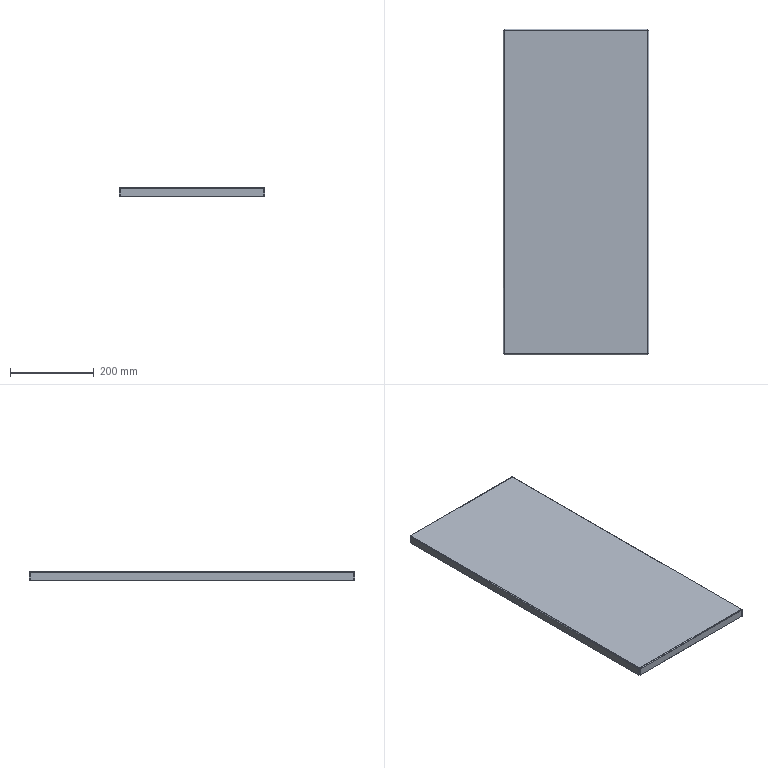Part | STEP file | X77-03015 | 1 solid | 38 faces | box 348 x 778 x 20 mm | volume 465951 mm3 | plane 22 | spline 8 | cylinder 8 | commonest cylinder face diameters 1.473 x4 4.473 x4